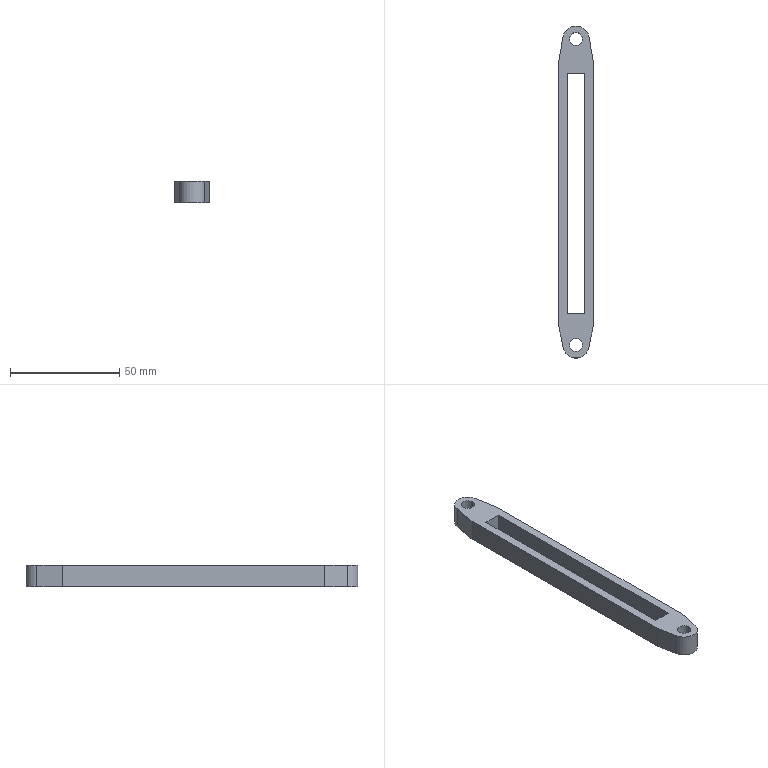Part | SolidWorks | features Extrusion 1 | 1 solid | 18 faces | box 16 x 152 x 10 mm | volume 13788 mm3 | plane 12 | cylinder 6 | commonest cylinder face diameters 6 x4 12 x2
STEP:
#1=CARTESIAN_POINT('',(5.,-9.303,10.));
#2=VERTEX_POINT('',#1);
#3=CARTESIAN_POINT('',(11.,-9.303,10.));
#4=VERTEX_POINT('',#3);
#5=CARTESIAN_POINT('',(8.,-9.303,10.));
#6=DIRECTION('',(0.,0.,1.));
#7=DIRECTION('',(1.,0.,0.));
#8=AXIS2_PLACEMENT_3D('',#5,#6,#7);
#9=CIRCLE('',#8,3.);
#10=EDGE_CURVE('',#2,#4,#9,.T.);
#11=ORIENTED_EDGE('',*,*,#10,.T.);
#12=CARTESIAN_POINT('',(11.,-9.303,0.));
#13=VERTEX_POINT('',#12);
#14=CARTESIAN_POINT('',(11.,-9.303,10.));
#15=DIRECTION('',(0.,0.,-1.));
#16=VECTOR('',#15,1000.);
#17=LINE('',#14,#16);
#18=EDGE_CURVE('',#4,#13,#17,.T.);
#19=ORIENTED_EDGE('',*,*,#18,.T.);
#20=CARTESIAN_POINT('',(5.,-9.303,0.));
#21=VERTEX_POINT('',#20);
#22=CARTESIAN_POINT('',(8.,-9.303,0.));
#23=DIRECTION('',(0.,0.,1.));
#24=DIRECTION('',(1.,0.,0.));
#25=AXIS2_PLACEMENT_3D('',#22,#23,#24);
#26=CIRCLE('',#25,3.);
#27=EDGE_CURVE('',#21,#13,#26,.T.);
#28=ORIENTED_EDGE('',*,*,#27,.F.);
#29=CARTESIAN_POINT('',(5.,-9.303,10.));
#30=DIRECTION('',(0.,0.,-1.));
#31=VECTOR('',#30,1000.);
#32=LINE('',#29,#31);
#33=EDGE_CURVE('',#2,#21,#32,.T.);
#34=ORIENTED_EDGE('',*,*,#33,.F.);
#35=EDGE_LOOP('',(#11,#19,#28,#34));
#36=FACE_OUTER_BOUND('',#35,.T.);
#37=CARTESIAN_POINT('',(8.,-9.303,10.));
#38=DIRECTION('',(0.,0.,-1.));
#39=DIRECTION('',(-1.,0.,0.));
#40=AXIS2_PLACEMENT_3D('',#37,#38,#39);
#41=CYLINDRICAL_SURFACE('',#40,3.);
#42=ADVANCED_FACE('',(#36),#41,.F.);
#43=CARTESIAN_POINT('',(5.,130.697,10.));
#44=VERTEX_POINT('',#43);
#45=CARTESIAN_POINT('',(11.,130.697,10.));
#46=VERTEX_POINT('',#45);
#47=CARTESIAN_POINT('',(8.,130.697,10.));
#48=DIRECTION('',(0.,0.,1.));
#49=DIRECTION('',(1.,0.,0.));
#50=AXIS2_PLACEMENT_3D('',#47,#48,#49);
#51=CIRCLE('',#50,3.);
#52=EDGE_CURVE('',#44,#46,#51,.T.);
#53=ORIENTED_EDGE('',*,*,#52,.T.);
#54=CARTESIAN_POINT('',(11.,130.697,0.));
#55=VERTEX_POINT('',#54);
#56=CARTESIAN_POINT('',(11.,130.697,10.));
#57=DIRECTION('',(0.,0.,-1.));
#58=VECTOR('',#57,1000.);
#59=LINE('',#56,#58);
#60=EDGE_CURVE('',#46,#55,#59,.T.);
#61=ORIENTED_EDGE('',*,*,#60,.T.);
#62=CARTESIAN_POINT('',(5.,130.697,0.));
#63=VERTEX_POINT('',#62);
#64=CARTESIAN_POINT('',(8.,130.697,0.));
#65=DIRECTION('',(0.,0.,1.));
#66=DIRECTION('',(1.,0.,0.));
#67=AXIS2_PLACEMENT_3D('',#64,#65,#66);
#68=CIRCLE('',#67,3.);
#69=EDGE_CURVE('',#63,#55,#68,.T.);
#70=ORIENTED_EDGE('',*,*,#69,.F.);
#71=CARTESIAN_POINT('',(5.,130.697,10.));
#72=DIRECTION('',(0.,0.,-1.));
#73=VECTOR('',#72,1000.);
#74=LINE('',#71,#73);
#75=EDGE_CURVE('',#44,#63,#74,.T.);
#76=ORIENTED_EDGE('',*,*,#75,.F.);
#77=EDGE_LOOP('',(#53,#61,#70,#76));
#78=FACE_OUTER_BOUND('',#77,.T.);
#79=CARTESIAN_POINT('',(8.,130.697,10.));
#80=DIRECTION('',(0.,0.,-1.));
#81=DIRECTION('',(-1.,0.,0.));
#82=AXIS2_PLACEMENT_3D('',#79,#80,#81);
#83=CYLINDRICAL_SURFACE('',#82,3.);
#84=ADVANCED_FACE('',(#78),#83,.F.);
#85=ORIENTED_EDGE('',*,*,#52,.F.);
#86=CARTESIAN_POINT('',(8.,130.697,10.));
#87=DIRECTION('',(0.,0.,1.));
#88=DIRECTION('',(1.,0.,0.));
#89=AXIS2_PLACEMENT_3D('',#86,#87,#88);
#90=CIRCLE('',#89,3.);
#91=EDGE_CURVE('',#46,#44,#90,.T.);
#92=ORIENTED_EDGE('',*,*,#91,.F.);
#93=EDGE_LOOP('',(#85,#92));
#94=FACE_BOUND('',#93,.T.);
#95=CARTESIAN_POINT('',(0.,120.,10.));
#96=VERTEX_POINT('',#95);
#97=CARTESIAN_POINT('',(0.,0.,10.));
#98=VERTEX_POINT('',#97);
#99=CARTESIAN_POINT('',(0.,0.,10.));
#100=DIRECTION('',(0.,-1.,0.));
#101=VECTOR('',#100,1000.);
#102=LINE('',#99,#101);
#103=EDGE_CURVE('',#96,#98,#102,.T.);
#104=ORIENTED_EDGE('',*,*,#103,.T.);
#105=CARTESIAN_POINT('',(2.119,-10.491,10.));
#106=VERTEX_POINT('',#105);
#107=CARTESIAN_POINT('',(2.119,-10.491,10.));
#108=DIRECTION('',(0.198,-0.9802,0.));
#109=VECTOR('',#108,1000.);
#110=LINE('',#107,#109);
#111=EDGE_CURVE('',#98,#106,#110,.T.);
#112=ORIENTED_EDGE('',*,*,#111,.T.);
#113=CARTESIAN_POINT('',(13.881,-10.491,10.));
#114=VERTEX_POINT('',#113);
#115=CARTESIAN_POINT('',(8.,-9.303,10.));
#116=DIRECTION('',(0.,0.,1.));
#117=DIRECTION('',(1.,0.,0.));
#118=AXIS2_PLACEMENT_3D('',#115,#116,#117);
#119=CIRCLE('',#118,6.);
#120=EDGE_CURVE('',#106,#114,#119,.T.);
#121=ORIENTED_EDGE('',*,*,#120,.T.);
#122=CARTESIAN_POINT('',(16.,0.,10.));
#123=VERTEX_POINT('',#122);
#124=CARTESIAN_POINT('',(16.,0.,10.));
#125=DIRECTION('',(0.198,0.9802,0.));
#126=VECTOR('',#125,1000.);
#127=LINE('',#124,#126);
#128=EDGE_CURVE('',#114,#123,#127,.T.);
#129=ORIENTED_EDGE('',*,*,#128,.T.);
#130=CARTESIAN_POINT('',(16.,120.,10.));
#131=VERTEX_POINT('',#130);
#132=CARTESIAN_POINT('',(16.,0.,10.));
#133=DIRECTION('',(0.,1.,0.));
#134=VECTOR('',#133,1000.);
#135=LINE('',#132,#134);
#136=EDGE_CURVE('',#123,#131,#135,.T.);
#137=ORIENTED_EDGE('',*,*,#136,.T.);
#138=CARTESIAN_POINT('',(13.907,131.749,10.));
#139=VERTEX_POINT('',#138);
#140=CARTESIAN_POINT('',(16.,120.,10.));
#141=DIRECTION('',(-0.1754,0.9845,0.));
#142=VECTOR('',#141,1000.);
#143=LINE('',#140,#142);
#144=EDGE_CURVE('',#131,#139,#143,.T.);
#145=ORIENTED_EDGE('',*,*,#144,.T.);
#146=CARTESIAN_POINT('',(2.093,131.749,10.));
#147=VERTEX_POINT('',#146);
#148=CARTESIAN_POINT('',(8.,130.697,10.));
#149=DIRECTION('',(0.,0.,1.));
#150=DIRECTION('',(1.,0.,0.));
#151=AXIS2_PLACEMENT_3D('',#148,#149,#150);
#152=CIRCLE('',#151,6.);
#153=EDGE_CURVE('',#139,#147,#152,.T.);
#154=ORIENTED_EDGE('',*,*,#153,.T.);
#155=CARTESIAN_POINT('',(0.,120.,10.));
#156=DIRECTION('',(-0.1754,-0.9845,0.));
#157=VECTOR('',#156,1000.);
#158=LINE('',#155,#157);
#159=EDGE_CURVE('',#147,#96,#158,.T.);
#160=ORIENTED_EDGE('',*,*,#159,.T.);
#161=EDGE_LOOP('',(#104,#112,#121,#129,#137,#145,#154,#160));
#162=FACE_OUTER_BOUND('',#161,.T.);
#163=CARTESIAN_POINT('',(4.,5.,10.));
#164=VERTEX_POINT('',#163);
#165=CARTESIAN_POINT('',(12.,5.,10.));
#166=VERTEX_POINT('',#165);
#167=CARTESIAN_POINT('',(4.,5.,10.));
#168=DIRECTION('',(1.,0.,0.));
#169=VECTOR('',#168,1000.);
#170=LINE('',#167,#169);
#171=EDGE_CURVE('',#164,#166,#170,.T.);
#172=ORIENTED_EDGE('',*,*,#171,.F.);
#173=CARTESIAN_POINT('',(4.,115.,10.));
#174=VERTEX_POINT('',#173);
#175=CARTESIAN_POINT('',(4.,115.,10.));
#176=DIRECTION('',(0.,-1.,0.));
#177=VECTOR('',#176,1000.);
#178=LINE('',#175,#177);
#179=EDGE_CURVE('',#174,#164,#178,.T.);
#180=ORIENTED_EDGE('',*,*,#179,.F.);
#181=CARTESIAN_POINT('',(12.,115.,10.));
#182=VERTEX_POINT('',#181);
#183=CARTESIAN_POINT('',(4.,115.,10.));
#184=DIRECTION('',(-1.,0.,0.));
#185=VECTOR('',#184,1000.);
#186=LINE('',#183,#185);
#187=EDGE_CURVE('',#182,#174,#186,.T.);
#188=ORIENTED_EDGE('',*,*,#187,.F.);
#189=CARTESIAN_POINT('',(12.,115.,10.));
#190=DIRECTION('',(0.,1.,0.));
#191=VECTOR('',#190,1000.);
#192=LINE('',#189,#191);
#193=EDGE_CURVE('',#166,#182,#192,.T.);
#194=ORIENTED_EDGE('',*,*,#193,.F.);
#195=EDGE_LOOP('',(#172,#180,#188,#194));
#196=FACE_BOUND('',#195,.T.);
#197=ORIENTED_EDGE('',*,*,#10,.F.);
#198=CARTESIAN_POINT('',(8.,-9.303,10.));
#199=DIRECTION('',(0.,0.,1.));
#200=DIRECTION('',(1.,0.,0.));
#201=AXIS2_PLACEMENT_3D('',#198,#199,#200);
#202=CIRCLE('',#201,3.);
#203=EDGE_CURVE('',#4,#2,#202,.T.);
#204=ORIENTED_EDGE('',*,*,#203,.F.);
#205=EDGE_LOOP('',(#197,#204));
#206=FACE_BOUND('',#205,.T.);
#207=CARTESIAN_POINT('',(8.,130.697,10.));
#208=DIRECTION('',(0.,0.,1.));
#209=DIRECTION('',(1.,0.,0.));
#210=AXIS2_PLACEMENT_3D('',#207,#208,#209);
#211=PLANE('',#210);
#212=ADVANCED_FACE('',(#94,#162,#196,#206),#211,.T.);
#213=CARTESIAN_POINT('',(0.,120.,0.));
#214=VERTEX_POINT('',#213);
#215=CARTESIAN_POINT('',(0.,0.,0.));
#216=VERTEX_POINT('',#215);
#217=CARTESIAN_POINT('',(0.,0.,0.));
#218=DIRECTION('',(0.,-1.,0.));
#219=VECTOR('',#218,1000.);
#220=LINE('',#217,#219);
#221=EDGE_CURVE('',#214,#216,#220,.T.);
#222=ORIENTED_EDGE('',*,*,#221,.F.);
#223=CARTESIAN_POINT('',(2.093,131.749,0.));
#224=VERTEX_POINT('',#223);
#225=CARTESIAN_POINT('',(0.,120.,0.));
#226=DIRECTION('',(-0.1754,-0.9845,0.));
#227=VECTOR('',#226,1000.);
#228=LINE('',#225,#227);
#229=EDGE_CURVE('',#224,#214,#228,.T.);
#230=ORIENTED_EDGE('',*,*,#229,.F.);
#231=CARTESIAN_POINT('',(13.907,131.749,0.));
#232=VERTEX_POINT('',#231);
#233=CARTESIAN_POINT('',(8.,130.697,0.));
#234=DIRECTION('',(0.,0.,1.));
#235=DIRECTION('',(1.,0.,0.));
#236=AXIS2_PLACEMENT_3D('',#233,#234,#235);
#237=CIRCLE('',#236,6.);
#238=EDGE_CURVE('',#232,#224,#237,.T.);
#239=ORIENTED_EDGE('',*,*,#238,.F.);
#240=CARTESIAN_POINT('',(16.,120.,0.));
#241=VERTEX_POINT('',#240);
#242=CARTESIAN_POINT('',(16.,120.,0.));
#243=DIRECTION('',(-0.1754,0.9845,0.));
#244=VECTOR('',#243,1000.);
#245=LINE('',#242,#244);
#246=EDGE_CURVE('',#241,#232,#245,.T.);
#247=ORIENTED_EDGE('',*,*,#246,.F.);
#248=CARTESIAN_POINT('',(16.,0.,0.));
#249=VERTEX_POINT('',#248);
#250=CARTESIAN_POINT('',(16.,0.,0.));
#251=DIRECTION('',(0.,1.,0.));
#252=VECTOR('',#251,1000.);
#253=LINE('',#250,#252);
#254=EDGE_CURVE('',#249,#241,#253,.T.);
#255=ORIENTED_EDGE('',*,*,#254,.F.);
#256=CARTESIAN_POINT('',(13.881,-10.491,0.));
#257=VERTEX_POINT('',#256);
#258=CARTESIAN_POINT('',(16.,0.,0.));
#259=DIRECTION('',(0.198,0.9802,0.));
#260=VECTOR('',#259,1000.);
#261=LINE('',#258,#260);
#262=EDGE_CURVE('',#257,#249,#261,.T.);
#263=ORIENTED_EDGE('',*,*,#262,.F.);
#264=CARTESIAN_POINT('',(2.119,-10.491,0.));
#265=VERTEX_POINT('',#264);
#266=CARTESIAN_POINT('',(8.,-9.303,0.));
#267=DIRECTION('',(0.,0.,1.));
#268=DIRECTION('',(1.,0.,0.));
#269=AXIS2_PLACEMENT_3D('',#266,#267,#268);
#270=CIRCLE('',#269,6.);
#271=EDGE_CURVE('',#265,#257,#270,.T.);
#272=ORIENTED_EDGE('',*,*,#271,.F.);
#273=CARTESIAN_POINT('',(2.119,-10.491,0.));
#274=DIRECTION('',(0.198,-0.9802,0.));
#275=VECTOR('',#274,1000.);
#276=LINE('',#273,#275);
#277=EDGE_CURVE('',#216,#265,#276,.T.);
#278=ORIENTED_EDGE('',*,*,#277,.F.);
#279=EDGE_LOOP('',(#222,#230,#239,#247,#255,#263,#272,#278));
#280=FACE_OUTER_BOUND('',#279,.T.);
#281=CARTESIAN_POINT('',(4.,115.,0.));
#282=VERTEX_POINT('',#281);
#283=CARTESIAN_POINT('',(4.,5.,0.));
#284=VERTEX_POINT('',#283);
#285=CARTESIAN_POINT('',(4.,115.,0.));
#286=DIRECTION('',(0.,-1.,0.));
#287=VECTOR('',#286,1000.);
#288=LINE('',#285,#287);
#289=EDGE_CURVE('',#282,#284,#288,.T.);
#290=ORIENTED_EDGE('',*,*,#289,.T.);
#291=CARTESIAN_POINT('',(12.,5.,0.));
#292=VERTEX_POINT('',#291);
#293=CARTESIAN_POINT('',(4.,5.,0.));
#294=DIRECTION('',(1.,0.,0.));
#295=VECTOR('',#294,1000.);
#296=LINE('',#293,#295);
#297=EDGE_CURVE('',#284,#292,#296,.T.);
#298=ORIENTED_EDGE('',*,*,#297,.T.);
#299=CARTESIAN_POINT('',(12.,115.,0.));
#300=VERTEX_POINT('',#299);
#301=CARTESIAN_POINT('',(12.,115.,0.));
#302=DIRECTION('',(0.,1.,0.));
#303=VECTOR('',#302,1000.);
#304=LINE('',#301,#303);
#305=EDGE_CURVE('',#292,#300,#304,.T.);
#306=ORIENTED_EDGE('',*,*,#305,.T.);
#307=CARTESIAN_POINT('',(4.,115.,0.));
#308=DIRECTION('',(-1.,0.,0.));
#309=VECTOR('',#308,1000.);
#310=LINE('',#307,#309);
#311=EDGE_CURVE('',#300,#282,#310,.T.);
#312=ORIENTED_EDGE('',*,*,#311,.T.);
#313=EDGE_LOOP('',(#290,#298,#306,#312));
#314=FACE_BOUND('',#313,.T.);
#315=ORIENTED_EDGE('',*,*,#69,.T.);
#316=CARTESIAN_POINT('',(8.,130.697,0.));
#317=DIRECTION('',(0.,0.,1.));
#318=DIRECTION('',(1.,0.,0.));
#319=AXIS2_PLACEMENT_3D('',#316,#317,#318);
#320=CIRCLE('',#319,3.);
#321=EDGE_CURVE('',#55,#63,#320,.T.);
#322=ORIENTED_EDGE('',*,*,#321,.T.);
#323=EDGE_LOOP('',(#315,#322));
#324=FACE_BOUND('',#323,.T.);
#325=ORIENTED_EDGE('',*,*,#27,.T.);
#326=CARTESIAN_POINT('',(8.,-9.303,0.));
#327=DIRECTION('',(0.,0.,1.));
#328=DIRECTION('',(1.,0.,0.));
#329=AXIS2_PLACEMENT_3D('',#326,#327,#328);
#330=CIRCLE('',#329,3.);
#331=EDGE_CURVE('',#13,#21,#330,.T.);
#332=ORIENTED_EDGE('',*,*,#331,.T.);
#333=EDGE_LOOP('',(#325,#332));
#334=FACE_BOUND('',#333,.T.);
#335=CARTESIAN_POINT('',(8.,130.697,0.));
#336=DIRECTION('',(0.,0.,1.));
#337=DIRECTION('',(1.,0.,0.));
#338=AXIS2_PLACEMENT_3D('',#335,#336,#337);
#339=PLANE('',#338);
#340=ADVANCED_FACE('',(#280,#314,#324,#334),#339,.F.);
#341=ORIENTED_EDGE('',*,*,#221,.T.);
#342=CARTESIAN_POINT('',(0.,0.,10.));
#343=DIRECTION('',(0.,0.,-1.));
#344=VECTOR('',#343,1000.);
#345=LINE('',#342,#344);
#346=EDGE_CURVE('',#98,#216,#345,.T.);
#347=ORIENTED_EDGE('',*,*,#346,.F.);
#348=ORIENTED_EDGE('',*,*,#103,.F.);
#349=CARTESIAN_POINT('',(0.,120.,10.));
#350=DIRECTION('',(0.,0.,-1.));
#351=VECTOR('',#350,1000.);
#352=LINE('',#349,#351);
#353=EDGE_CURVE('',#96,#214,#352,.T.);
#354=ORIENTED_EDGE('',*,*,#353,.T.);
#355=EDGE_LOOP('',(#341,#347,#348,#354));
#356=FACE_OUTER_BOUND('',#355,.T.);
#357=CARTESIAN_POINT('',(0.,0.,10.));
#358=DIRECTION('',(1.,0.,0.));
#359=DIRECTION('',(0.,0.,-1.));
#360=AXIS2_PLACEMENT_3D('',#357,#358,#359);
#361=PLANE('',#360);
#362=ADVANCED_FACE('',(#356),#361,.F.);
#363=ORIENTED_EDGE('',*,*,#277,.T.);
#364=CARTESIAN_POINT('',(2.119,-10.491,10.));
#365=DIRECTION('',(0.,0.,-1.));
#366=VECTOR('',#365,1000.);
#367=LINE('',#364,#366);
#368=EDGE_CURVE('',#106,#265,#367,.T.);
#369=ORIENTED_EDGE('',*,*,#368,.F.);
#370=ORIENTED_EDGE('',*,*,#111,.F.);
#371=ORIENTED_EDGE('',*,*,#346,.T.);
#372=EDGE_LOOP('',(#363,#369,#370,#371));
#373=FACE_OUTER_BOUND('',#372,.T.);
#374=CARTESIAN_POINT('',(2.119,-10.491,10.));
#375=DIRECTION('',(0.9802,0.198,0.));
#376=DIRECTION('',(-0.198,0.9802,0.));
#377=AXIS2_PLACEMENT_3D('',#374,#375,#376);
#378=PLANE('',#377);
#379=ADVANCED_FACE('',(#373),#378,.F.);
#380=ORIENTED_EDGE('',*,*,#271,.T.);
#381=CARTESIAN_POINT('',(13.881,-10.491,10.));
#382=DIRECTION('',(0.,0.,-1.));
#383=VECTOR('',#382,1000.);
#384=LINE('',#381,#383);
#385=EDGE_CURVE('',#114,#257,#384,.T.);
#386=ORIENTED_EDGE('',*,*,#385,.F.);
#387=ORIENTED_EDGE('',*,*,#120,.F.);
#388=ORIENTED_EDGE('',*,*,#368,.T.);
#389=EDGE_LOOP('',(#380,#386,#387,#388));
#390=FACE_OUTER_BOUND('',#389,.T.);
#391=CARTESIAN_POINT('',(8.,-9.303,10.));
#392=DIRECTION('',(0.,0.,-1.));
#393=DIRECTION('',(-1.,0.,0.));
#394=AXIS2_PLACEMENT_3D('',#391,#392,#393);
#395=CYLINDRICAL_SURFACE('',#394,6.);
#396=ADVANCED_FACE('',(#390),#395,.T.);
#397=ORIENTED_EDGE('',*,*,#262,.T.);
#398=CARTESIAN_POINT('',(16.,0.,10.));
#399=DIRECTION('',(0.,0.,-1.));
#400=VECTOR('',#399,1000.);
#401=LINE('',#398,#400);
#402=EDGE_CURVE('',#123,#249,#401,.T.);
#403=ORIENTED_EDGE('',*,*,#402,.F.);
#404=ORIENTED_EDGE('',*,*,#128,.F.);
#405=ORIENTED_EDGE('',*,*,#385,.T.);
#406=EDGE_LOOP('',(#397,#403,#404,#405));
#407=FACE_OUTER_BOUND('',#406,.T.);
#408=CARTESIAN_POINT('',(16.,0.,10.));
#409=DIRECTION('',(-0.9802,0.198,0.));
#410=DIRECTION('',(-0.198,-0.9802,0.));
#411=AXIS2_PLACEMENT_3D('',#408,#409,#410);
#412=PLANE('',#411);
#413=ADVANCED_FACE('',(#407),#412,.F.);
#414=ORIENTED_EDGE('',*,*,#254,.T.);
#415=CARTESIAN_POINT('',(16.,120.,10.));
#416=DIRECTION('',(0.,0.,-1.));
#417=VECTOR('',#416,1000.);
#418=LINE('',#415,#417);
#419=EDGE_CURVE('',#131,#241,#418,.T.);
#420=ORIENTED_EDGE('',*,*,#419,.F.);
#421=ORIENTED_EDGE('',*,*,#136,.F.);
#422=ORIENTED_EDGE('',*,*,#402,.T.);
#423=EDGE_LOOP('',(#414,#420,#421,#422));
#424=FACE_OUTER_BOUND('',#423,.T.);
#425=CARTESIAN_POINT('',(16.,0.,10.));
#426=DIRECTION('',(-1.,0.,0.));
#427=DIRECTION('',(0.,0.,1.));
#428=AXIS2_PLACEMENT_3D('',#425,#426,#427);
#429=PLANE('',#428);
#430=ADVANCED_FACE('',(#424),#429,.F.);
#431=ORIENTED_EDGE('',*,*,#246,.T.);
#432=CARTESIAN_POINT('',(13.907,131.749,10.));
#433=DIRECTION('',(0.,0.,-1.));
#434=VECTOR('',#433,1000.);
#435=LINE('',#432,#434);
#436=EDGE_CURVE('',#139,#232,#435,.T.);
#437=ORIENTED_EDGE('',*,*,#436,.F.);
#438=ORIENTED_EDGE('',*,*,#144,.F.);
#439=ORIENTED_EDGE('',*,*,#419,.T.);
#440=EDGE_LOOP('',(#431,#437,#438,#439));
#441=FACE_OUTER_BOUND('',#440,.T.);
#442=CARTESIAN_POINT('',(16.,120.,10.));
#443=DIRECTION('',(-0.9845,-0.1754,0.));
#444=DIRECTION('',(0.1754,-0.9845,0.));
#445=AXIS2_PLACEMENT_3D('',#442,#443,#444);
#446=PLANE('',#445);
#447=ADVANCED_FACE('',(#441),#446,.F.);
#448=ORIENTED_EDGE('',*,*,#238,.T.);
#449=CARTESIAN_POINT('',(2.093,131.749,10.));
#450=DIRECTION('',(0.,0.,-1.));
#451=VECTOR('',#450,1000.);
#452=LINE('',#449,#451);
#453=EDGE_CURVE('',#147,#224,#452,.T.);
#454=ORIENTED_EDGE('',*,*,#453,.F.);
#455=ORIENTED_EDGE('',*,*,#153,.F.);
#456=ORIENTED_EDGE('',*,*,#436,.T.);
#457=EDGE_LOOP('',(#448,#454,#455,#456));
#458=FACE_OUTER_BOUND('',#457,.T.);
#459=CARTESIAN_POINT('',(8.,130.697,10.));
#460=DIRECTION('',(0.,0.,-1.));
#461=DIRECTION('',(-1.,0.,0.));
#462=AXIS2_PLACEMENT_3D('',#459,#460,#461);
#463=CYLINDRICAL_SURFACE('',#462,6.);
#464=ADVANCED_FACE('',(#458),#463,.T.);
#465=ORIENTED_EDGE('',*,*,#229,.T.);
#466=ORIENTED_EDGE('',*,*,#353,.F.);
#467=ORIENTED_EDGE('',*,*,#159,.F.);
#468=ORIENTED_EDGE('',*,*,#453,.T.);
#469=EDGE_LOOP('',(#465,#466,#467,#468));
#470=FACE_OUTER_BOUND('',#469,.T.);
#471=CARTESIAN_POINT('',(0.,120.,10.));
#472=DIRECTION('',(0.9845,-0.1754,0.));
#473=DIRECTION('',(0.1754,0.9845,0.));
#474=AXIS2_PLACEMENT_3D('',#471,#472,#473);
#475=PLANE('',#474);
#476=ADVANCED_FACE('',(#470),#475,.F.);
#477=ORIENTED_EDGE('',*,*,#289,.F.);
#478=CARTESIAN_POINT('',(4.,115.,10.));
#479=DIRECTION('',(0.,0.,-1.));
#480=VECTOR('',#479,1000.);
#481=LINE('',#478,#480);
#482=EDGE_CURVE('',#174,#282,#481,.T.);
#483=ORIENTED_EDGE('',*,*,#482,.F.);
#484=ORIENTED_EDGE('',*,*,#179,.T.);
#485=CARTESIAN_POINT('',(4.,5.,10.));
#486=DIRECTION('',(0.,0.,-1.));
#487=VECTOR('',#486,1000.);
#488=LINE('',#485,#487);
#489=EDGE_CURVE('',#164,#284,#488,.T.);
#490=ORIENTED_EDGE('',*,*,#489,.T.);
#491=EDGE_LOOP('',(#477,#483,#484,#490));
#492=FACE_OUTER_BOUND('',#491,.T.);
#493=CARTESIAN_POINT('',(4.,115.,10.));
#494=DIRECTION('',(1.,0.,0.));
#495=DIRECTION('',(0.,1.,0.));
#496=AXIS2_PLACEMENT_3D('',#493,#494,#495);
#497=PLANE('',#496);
#498=ADVANCED_FACE('',(#492),#497,.T.);
#499=ORIENTED_EDGE('',*,*,#297,.F.);
#500=ORIENTED_EDGE('',*,*,#489,.F.);
#501=ORIENTED_EDGE('',*,*,#171,.T.);
#502=CARTESIAN_POINT('',(12.,5.,10.));
#503=DIRECTION('',(0.,0.,-1.));
#504=VECTOR('',#503,1000.);
#505=LINE('',#502,#504);
#506=EDGE_CURVE('',#166,#292,#505,.T.);
#507=ORIENTED_EDGE('',*,*,#506,.T.);
#508=EDGE_LOOP('',(#499,#500,#501,#507));
#509=FACE_OUTER_BOUND('',#508,.T.);
#510=CARTESIAN_POINT('',(4.,5.,10.));
#511=DIRECTION('',(0.,1.,0.));
#512=DIRECTION('',(-1.,0.,0.));
#513=AXIS2_PLACEMENT_3D('',#510,#511,#512);
#514=PLANE('',#513);
#515=ADVANCED_FACE('',(#509),#514,.T.);
#516=ORIENTED_EDGE('',*,*,#305,.F.);
#517=ORIENTED_EDGE('',*,*,#506,.F.);
#518=ORIENTED_EDGE('',*,*,#193,.T.);
#519=CARTESIAN_POINT('',(12.,115.,10.));
#520=DIRECTION('',(0.,0.,-1.));
#521=VECTOR('',#520,1000.);
#522=LINE('',#519,#521);
#523=EDGE_CURVE('',#182,#300,#522,.T.);
#524=ORIENTED_EDGE('',*,*,#523,.T.);
#525=EDGE_LOOP('',(#516,#517,#518,#524));
#526=FACE_OUTER_BOUND('',#525,.T.);
#527=CARTESIAN_POINT('',(12.,115.,10.));
#528=DIRECTION('',(-1.,0.,0.));
#529=DIRECTION('',(0.,-1.,0.));
#530=AXIS2_PLACEMENT_3D('',#527,#528,#529);
#531=PLANE('',#530);
#532=ADVANCED_FACE('',(#526),#531,.T.);
#533=ORIENTED_EDGE('',*,*,#311,.F.);
#534=ORIENTED_EDGE('',*,*,#523,.F.);
#535=ORIENTED_EDGE('',*,*,#187,.T.);
#536=ORIENTED_EDGE('',*,*,#482,.T.);
#537=EDGE_LOOP('',(#533,#534,#535,#536));
#538=FACE_OUTER_BOUND('',#537,.T.);
#539=CARTESIAN_POINT('',(4.,115.,10.));
#540=DIRECTION('',(0.,-1.,0.));
#541=DIRECTION('',(0.,0.,-1.));
#542=AXIS2_PLACEMENT_3D('',#539,#540,#541);
#543=PLANE('',#542);
#544=ADVANCED_FACE('',(#538),#543,.T.);
#545=ORIENTED_EDGE('',*,*,#60,.F.);
#546=ORIENTED_EDGE('',*,*,#91,.T.);
#547=ORIENTED_EDGE('',*,*,#75,.T.);
#548=ORIENTED_EDGE('',*,*,#321,.F.);
#549=EDGE_LOOP('',(#545,#546,#547,#548));
#550=FACE_OUTER_BOUND('',#549,.T.);
#551=CARTESIAN_POINT('',(8.,130.697,10.));
#552=DIRECTION('',(0.,0.,-1.));
#553=DIRECTION('',(-1.,0.,0.));
#554=AXIS2_PLACEMENT_3D('',#551,#552,#553);
#555=CYLINDRICAL_SURFACE('',#554,3.);
#556=ADVANCED_FACE('',(#550),#555,.F.);
#557=ORIENTED_EDGE('',*,*,#18,.F.);
#558=ORIENTED_EDGE('',*,*,#203,.T.);
#559=ORIENTED_EDGE('',*,*,#33,.T.);
#560=ORIENTED_EDGE('',*,*,#331,.F.);
#561=EDGE_LOOP('',(#557,#558,#559,#560));
#562=FACE_OUTER_BOUND('',#561,.T.);
#563=CARTESIAN_POINT('',(8.,-9.303,10.));
#564=DIRECTION('',(0.,0.,-1.));
#565=DIRECTION('',(-1.,0.,0.));
#566=AXIS2_PLACEMENT_3D('',#563,#564,#565);
#567=CYLINDRICAL_SURFACE('',#566,3.);
#568=ADVANCED_FACE('',(#562),#567,.F.);
#569=CLOSED_SHELL('',(#42,#84,#212,#340,#362,#379,#396,#413,#430,#447,#464,#476,#498,#515,#532,#544,#556,#568));
#570=MANIFOLD_SOLID_BREP('',#569);
#571=CARTESIAN_POINT('',(0.,0.,0.));
#572=DIRECTION('',(0.,0.,1.));
#573=DIRECTION('',(1.,0.,0.));
#574=AXIS2_PLACEMENT_3D('',#571,#572,#573);
#575=(LENGTH_UNIT()NAMED_UNIT(*)SI_UNIT(.MILLI.,.METRE.));
#576=UNCERTAINTY_MEASURE_WITH_UNIT(LENGTH_MEASURE(0.00001),#575,'','');
#577=(NAMED_UNIT(*)PLANE_ANGLE_UNIT()SI_UNIT($,.RADIAN.));
#578=(NAMED_UNIT(*)SI_UNIT($,.STERADIAN.)SOLID_ANGLE_UNIT());
#579=(GEOMETRIC_REPRESENTATION_CONTEXT(3)GLOBAL_UNCERTAINTY_ASSIGNED_CONTEXT((#576))GLOBAL_UNIT_ASSIGNED_CONTEXT((#575,#577,#578))REPRESENTATION_CONTEXT('',''));
#580=ADVANCED_BREP_SHAPE_REPRESENTATION('',(#570,#574),#579);